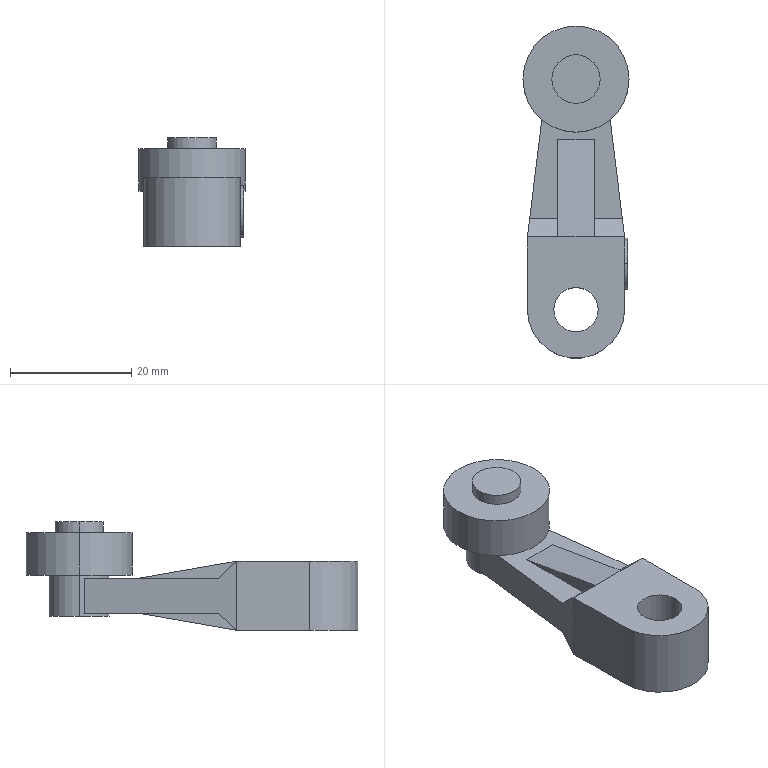Part | SolidWorks | features BaseBody 1 | 1 solid | 34 faces | box 17.5 x 54.75 x 17.9 mm | volume 7250 mm3 | plane 23 | cylinder 11 | commonest cylinder face diameters 7.3 x2 8 x2 8.5 x2 10 x2 17.5 x2 16 x1
STEP:
#1=CARTESIAN_POINT('',(-3.65,0.,0.));
#2=VERTEX_POINT('',#1);
#3=CARTESIAN_POINT('',(3.65,0.,0.));
#4=VERTEX_POINT('',#3);
#5=CARTESIAN_POINT('',(0.,0.,0.));
#6=DIRECTION('',(0.,0.,1.));
#7=DIRECTION('',(1.,0.,0.));
#8=AXIS2_PLACEMENT_3D('',#5,#6,#7);
#9=CIRCLE('',#8,3.65);
#10=EDGE_CURVE('',#2,#4,#9,.T.);
#11=ORIENTED_EDGE('',*,*,#10,.F.);
#12=CARTESIAN_POINT('',(-3.65,0.,11.4));
#13=VERTEX_POINT('',#12);
#14=CARTESIAN_POINT('',(-3.65,0.,0.));
#15=DIRECTION('',(0.,0.,1.));
#16=VECTOR('',#15,1000.);
#17=LINE('',#14,#16);
#18=EDGE_CURVE('',#2,#13,#17,.T.);
#19=ORIENTED_EDGE('',*,*,#18,.T.);
#20=CARTESIAN_POINT('',(3.65,0.,11.4));
#21=VERTEX_POINT('',#20);
#22=CARTESIAN_POINT('',(0.,0.,11.4));
#23=DIRECTION('',(0.,0.,1.));
#24=DIRECTION('',(1.,0.,0.));
#25=AXIS2_PLACEMENT_3D('',#22,#23,#24);
#26=CIRCLE('',#25,3.65);
#27=EDGE_CURVE('',#13,#21,#26,.T.);
#28=ORIENTED_EDGE('',*,*,#27,.T.);
#29=CARTESIAN_POINT('',(3.65,0.,0.));
#30=DIRECTION('',(0.,0.,1.));
#31=VECTOR('',#30,1000.);
#32=LINE('',#29,#31);
#33=EDGE_CURVE('',#4,#21,#32,.T.);
#34=ORIENTED_EDGE('',*,*,#33,.F.);
#35=EDGE_LOOP('',(#11,#19,#28,#34));
#36=FACE_OUTER_BOUND('',#35,.T.);
#37=CARTESIAN_POINT('',(0.,0.,0.));
#38=DIRECTION('',(0.,0.,1.));
#39=DIRECTION('',(1.,0.,0.));
#40=AXIS2_PLACEMENT_3D('',#37,#38,#39);
#41=CYLINDRICAL_SURFACE('',#40,3.65);
#42=ADVANCED_FACE('',(#36),#41,.F.);
#43=CARTESIAN_POINT('',(8.5,7.6,1.45));
#44=VERTEX_POINT('',#43);
#45=CARTESIAN_POINT('',(8.5,7.6,9.95));
#46=VERTEX_POINT('',#45);
#47=CARTESIAN_POINT('',(8.5,7.6,5.7));
#48=DIRECTION('',(1.,0.,0.));
#49=DIRECTION('',(0.,0.,-1.));
#50=AXIS2_PLACEMENT_3D('',#47,#48,#49);
#51=CIRCLE('',#50,4.25);
#52=EDGE_CURVE('',#44,#46,#51,.T.);
#53=ORIENTED_EDGE('',*,*,#52,.F.);
#54=CARTESIAN_POINT('',(8.,7.6,1.45));
#55=VERTEX_POINT('',#54);
#56=CARTESIAN_POINT('',(8.5,7.6,1.45));
#57=DIRECTION('',(-1.,0.,0.));
#58=VECTOR('',#57,1000.);
#59=LINE('',#56,#58);
#60=EDGE_CURVE('',#44,#55,#59,.T.);
#61=ORIENTED_EDGE('',*,*,#60,.T.);
#62=CARTESIAN_POINT('',(8.,7.6,9.95));
#63=VERTEX_POINT('',#62);
#64=CARTESIAN_POINT('',(8.,7.6,5.7));
#65=DIRECTION('',(1.,0.,0.));
#66=DIRECTION('',(0.,0.,-1.));
#67=AXIS2_PLACEMENT_3D('',#64,#65,#66);
#68=CIRCLE('',#67,4.25);
#69=EDGE_CURVE('',#55,#63,#68,.T.);
#70=ORIENTED_EDGE('',*,*,#69,.T.);
#71=CARTESIAN_POINT('',(8.5,7.6,9.95));
#72=DIRECTION('',(-1.,0.,0.));
#73=VECTOR('',#72,1000.);
#74=LINE('',#71,#73);
#75=EDGE_CURVE('',#46,#63,#74,.T.);
#76=ORIENTED_EDGE('',*,*,#75,.F.);
#77=EDGE_LOOP('',(#53,#61,#70,#76));
#78=FACE_OUTER_BOUND('',#77,.T.);
#79=CARTESIAN_POINT('',(8.5,7.6,5.7));
#80=DIRECTION('',(-1.,0.,0.));
#81=DIRECTION('',(0.,0.,1.));
#82=AXIS2_PLACEMENT_3D('',#79,#80,#81);
#83=CYLINDRICAL_SURFACE('',#82,4.25);
#84=ADVANCED_FACE('',(#78),#83,.T.);
#85=CARTESIAN_POINT('',(4.,38.,17.9));
#86=VERTEX_POINT('',#85);
#87=CARTESIAN_POINT('',(-4.,38.,17.9));
#88=VERTEX_POINT('',#87);
#89=CARTESIAN_POINT('',(0.,38.,17.9));
#90=DIRECTION('',(0.,0.,1.));
#91=DIRECTION('',(1.,0.,0.));
#92=AXIS2_PLACEMENT_3D('',#89,#90,#91);
#93=CIRCLE('',#92,4.);
#94=EDGE_CURVE('',#86,#88,#93,.T.);
#95=ORIENTED_EDGE('',*,*,#94,.F.);
#96=CARTESIAN_POINT('',(4.,38.,16.1));
#97=VERTEX_POINT('',#96);
#98=CARTESIAN_POINT('',(4.,38.,17.9));
#99=DIRECTION('',(0.,0.,-1.));
#100=VECTOR('',#99,1000.);
#101=LINE('',#98,#100);
#102=EDGE_CURVE('',#86,#97,#101,.T.);
#103=ORIENTED_EDGE('',*,*,#102,.T.);
#104=CARTESIAN_POINT('',(-4.,38.,16.1));
#105=VERTEX_POINT('',#104);
#106=CARTESIAN_POINT('',(0.,38.,16.1));
#107=DIRECTION('',(0.,0.,1.));
#108=DIRECTION('',(1.,0.,0.));
#109=AXIS2_PLACEMENT_3D('',#106,#107,#108);
#110=CIRCLE('',#109,4.);
#111=EDGE_CURVE('',#97,#105,#110,.T.);
#112=ORIENTED_EDGE('',*,*,#111,.T.);
#113=CARTESIAN_POINT('',(-4.,38.,17.9));
#114=DIRECTION('',(0.,0.,-1.));
#115=VECTOR('',#114,1000.);
#116=LINE('',#113,#115);
#117=EDGE_CURVE('',#88,#105,#116,.T.);
#118=ORIENTED_EDGE('',*,*,#117,.F.);
#119=EDGE_LOOP('',(#95,#103,#112,#118));
#120=FACE_OUTER_BOUND('',#119,.T.);
#121=CARTESIAN_POINT('',(0.,38.,17.9));
#122=DIRECTION('',(0.,0.,-1.));
#123=DIRECTION('',(-1.,0.,0.));
#124=AXIS2_PLACEMENT_3D('',#121,#122,#123);
#125=CYLINDRICAL_SURFACE('',#124,4.);
#126=ADVANCED_FACE('',(#120),#125,.T.);
#127=CARTESIAN_POINT('',(8.75,38.,16.1));
#128=VERTEX_POINT('',#127);
#129=CARTESIAN_POINT('',(-8.75,38.,16.1));
#130=VERTEX_POINT('',#129);
#131=CARTESIAN_POINT('',(0.,38.,16.1));
#132=DIRECTION('',(0.,0.,1.));
#133=DIRECTION('',(1.,0.,0.));
#134=AXIS2_PLACEMENT_3D('',#131,#132,#133);
#135=CIRCLE('',#134,8.75);
#136=EDGE_CURVE('',#128,#130,#135,.T.);
#137=ORIENTED_EDGE('',*,*,#136,.F.);
#138=CARTESIAN_POINT('',(8.75,38.,9.1));
#139=VERTEX_POINT('',#138);
#140=CARTESIAN_POINT('',(8.75,38.,16.1));
#141=DIRECTION('',(0.,0.,-1.));
#142=VECTOR('',#141,1000.);
#143=LINE('',#140,#142);
#144=EDGE_CURVE('',#128,#139,#143,.T.);
#145=ORIENTED_EDGE('',*,*,#144,.T.);
#146=CARTESIAN_POINT('',(-8.75,38.,9.1));
#147=VERTEX_POINT('',#146);
#148=CARTESIAN_POINT('',(0.,38.,9.1));
#149=DIRECTION('',(0.,0.,1.));
#150=DIRECTION('',(1.,0.,0.));
#151=AXIS2_PLACEMENT_3D('',#148,#149,#150);
#152=CIRCLE('',#151,8.75);
#153=EDGE_CURVE('',#139,#147,#152,.T.);
#154=ORIENTED_EDGE('',*,*,#153,.T.);
#155=CARTESIAN_POINT('',(-8.75,38.,16.1));
#156=DIRECTION('',(0.,0.,-1.));
#157=VECTOR('',#156,1000.);
#158=LINE('',#155,#157);
#159=EDGE_CURVE('',#130,#147,#158,.T.);
#160=ORIENTED_EDGE('',*,*,#159,.F.);
#161=EDGE_LOOP('',(#137,#145,#154,#160));
#162=FACE_OUTER_BOUND('',#161,.T.);
#163=CARTESIAN_POINT('',(0.,38.,16.1));
#164=DIRECTION('',(0.,0.,-1.));
#165=DIRECTION('',(-1.,0.,0.));
#166=AXIS2_PLACEMENT_3D('',#163,#164,#165);
#167=CYLINDRICAL_SURFACE('',#166,8.75);
#168=ADVANCED_FACE('',(#162),#167,.T.);
#169=CARTESIAN_POINT('',(-5.,38.,2.3));
#170=VERTEX_POINT('',#169);
#171=CARTESIAN_POINT('',(5.,38.,2.3));
#172=VERTEX_POINT('',#171);
#173=CARTESIAN_POINT('',(0.,38.,2.3));
#174=DIRECTION('',(0.,0.,-1.));
#175=DIRECTION('',(-1.,0.,0.));
#176=AXIS2_PLACEMENT_3D('',#173,#174,#175);
#177=CIRCLE('',#176,5.);
#178=EDGE_CURVE('',#170,#172,#177,.T.);
#179=ORIENTED_EDGE('',*,*,#178,.F.);
#180=CARTESIAN_POINT('',(-5.,38.,9.1));
#181=VERTEX_POINT('',#180);
#182=CARTESIAN_POINT('',(-5.,38.,2.3));
#183=DIRECTION('',(0.,0.,1.));
#184=VECTOR('',#183,1000.);
#185=LINE('',#182,#184);
#186=EDGE_CURVE('',#170,#181,#185,.T.);
#187=ORIENTED_EDGE('',*,*,#186,.T.);
#188=CARTESIAN_POINT('',(5.,38.,9.1));
#189=VERTEX_POINT('',#188);
#190=CARTESIAN_POINT('',(0.,38.,9.1));
#191=DIRECTION('',(0.,0.,1.));
#192=DIRECTION('',(1.,0.,0.));
#193=AXIS2_PLACEMENT_3D('',#190,#191,#192);
#194=CIRCLE('',#193,5.);
#195=EDGE_CURVE('',#189,#181,#194,.T.);
#196=ORIENTED_EDGE('',*,*,#195,.F.);
#197=CARTESIAN_POINT('',(5.,38.,2.3));
#198=DIRECTION('',(0.,0.,1.));
#199=VECTOR('',#198,1000.);
#200=LINE('',#197,#199);
#201=EDGE_CURVE('',#172,#189,#200,.T.);
#202=ORIENTED_EDGE('',*,*,#201,.F.);
#203=EDGE_LOOP('',(#179,#187,#196,#202));
#204=FACE_OUTER_BOUND('',#203,.T.);
#205=CARTESIAN_POINT('',(0.,38.,2.3));
#206=DIRECTION('',(0.,0.,1.));
#207=DIRECTION('',(1.,0.,0.));
#208=AXIS2_PLACEMENT_3D('',#205,#206,#207);
#209=CYLINDRICAL_SURFACE('',#208,5.);
#210=ADVANCED_FACE('',(#204),#209,.T.);
#211=CARTESIAN_POINT('',(8.,0.,0.));
#212=VERTEX_POINT('',#211);
#213=CARTESIAN_POINT('',(8.,12.,0.));
#214=VERTEX_POINT('',#213);
#215=CARTESIAN_POINT('',(8.,0.,0.));
#216=DIRECTION('',(0.,1.,0.));
#217=VECTOR('',#216,1000.);
#218=LINE('',#215,#217);
#219=EDGE_CURVE('',#212,#214,#218,.T.);
#220=ORIENTED_EDGE('',*,*,#219,.T.);
#221=CARTESIAN_POINT('',(8.,12.,11.4));
#222=VERTEX_POINT('',#221);
#223=CARTESIAN_POINT('',(8.,12.,11.4));
#224=DIRECTION('',(0.,0.,1.));
#225=VECTOR('',#224,1000.);
#226=LINE('',#223,#225);
#227=EDGE_CURVE('',#214,#222,#226,.T.);
#228=ORIENTED_EDGE('',*,*,#227,.T.);
#229=CARTESIAN_POINT('',(8.,0.,11.4));
#230=VERTEX_POINT('',#229);
#231=CARTESIAN_POINT('',(8.,0.,11.4));
#232=DIRECTION('',(0.,-1.,0.));
#233=VECTOR('',#232,1000.);
#234=LINE('',#231,#233);
#235=EDGE_CURVE('',#222,#230,#234,.T.);
#236=ORIENTED_EDGE('',*,*,#235,.T.);
#237=CARTESIAN_POINT('',(8.,0.,11.4));
#238=DIRECTION('',(0.,0.,-1.));
#239=VECTOR('',#238,1000.);
#240=LINE('',#237,#239);
#241=EDGE_CURVE('',#230,#212,#240,.T.);
#242=ORIENTED_EDGE('',*,*,#241,.T.);
#243=EDGE_LOOP('',(#220,#228,#236,#242));
#244=FACE_OUTER_BOUND('',#243,.T.);
#245=CARTESIAN_POINT('',(8.,7.6,5.7));
#246=DIRECTION('',(1.,0.,0.));
#247=DIRECTION('',(0.,0.,-1.));
#248=AXIS2_PLACEMENT_3D('',#245,#246,#247);
#249=CIRCLE('',#248,4.25);
#250=EDGE_CURVE('',#63,#55,#249,.T.);
#251=ORIENTED_EDGE('',*,*,#250,.F.);
#252=ORIENTED_EDGE('',*,*,#69,.F.);
#253=EDGE_LOOP('',(#251,#252));
#254=FACE_BOUND('',#253,.T.);
#255=CARTESIAN_POINT('',(8.,38.,11.4));
#256=DIRECTION('',(1.,0.,0.));
#257=DIRECTION('',(0.,0.,-1.));
#258=AXIS2_PLACEMENT_3D('',#255,#256,#257);
#259=PLANE('',#258);
#260=ADVANCED_FACE('',(#244,#254),#259,.T.);
#261=CARTESIAN_POINT('',(0.,38.,16.1));
#262=DIRECTION('',(0.,0.,1.));
#263=DIRECTION('',(1.,0.,0.));
#264=AXIS2_PLACEMENT_3D('',#261,#262,#263);
#265=CIRCLE('',#264,8.75);
#266=EDGE_CURVE('',#130,#128,#265,.T.);
#267=ORIENTED_EDGE('',*,*,#266,.T.);
#268=ORIENTED_EDGE('',*,*,#136,.T.);
#269=EDGE_LOOP('',(#267,#268));
#270=FACE_OUTER_BOUND('',#269,.T.);
#271=CARTESIAN_POINT('',(0.,38.,16.1));
#272=DIRECTION('',(0.,0.,1.));
#273=DIRECTION('',(1.,0.,0.));
#274=AXIS2_PLACEMENT_3D('',#271,#272,#273);
#275=CIRCLE('',#274,4.);
#276=EDGE_CURVE('',#105,#97,#275,.T.);
#277=ORIENTED_EDGE('',*,*,#276,.F.);
#278=ORIENTED_EDGE('',*,*,#111,.F.);
#279=EDGE_LOOP('',(#277,#278));
#280=FACE_BOUND('',#279,.T.);
#281=CARTESIAN_POINT('',(0.,38.,16.1));
#282=DIRECTION('',(0.,0.,1.));
#283=DIRECTION('',(1.,0.,0.));
#284=AXIS2_PLACEMENT_3D('',#281,#282,#283);
#285=PLANE('',#284);
#286=ADVANCED_FACE('',(#270,#280),#285,.T.);
#287=CARTESIAN_POINT('',(-7.632,15.,2.8));
#288=VERTEX_POINT('',#287);
#289=CARTESIAN_POINT('',(-3.,15.,2.8));
#290=VERTEX_POINT('',#289);
#291=CARTESIAN_POINT('',(-8.,15.,2.8));
#292=DIRECTION('',(1.,0.,0.));
#293=VECTOR('',#292,1000.);
#294=LINE('',#291,#293);
#295=EDGE_CURVE('',#288,#290,#294,.T.);
#296=ORIENTED_EDGE('',*,*,#295,.T.);
#297=CARTESIAN_POINT('',(-3.,12.,0.));
#298=VERTEX_POINT('',#297);
#299=CARTESIAN_POINT('',(-3.,15.,2.8));
#300=DIRECTION('',(0.,-0.7311,-0.6823));
#301=VECTOR('',#300,1000.);
#302=LINE('',#299,#301);
#303=EDGE_CURVE('',#290,#298,#302,.T.);
#304=ORIENTED_EDGE('',*,*,#303,.T.);
#305=CARTESIAN_POINT('',(-8.,12.,0.));
#306=VERTEX_POINT('',#305);
#307=CARTESIAN_POINT('',(-8.,12.,0.));
#308=DIRECTION('',(1.,0.,0.));
#309=VECTOR('',#308,1000.);
#310=LINE('',#307,#309);
#311=EDGE_CURVE('',#306,#298,#310,.T.);
#312=ORIENTED_EDGE('',*,*,#311,.F.);
#313=CARTESIAN_POINT('',(-7.635,14.976,2.778));
#314=DIRECTION('',(0.0894,0.7281,0.6796));
#315=VECTOR('',#314,1000.);
#316=LINE('',#313,#315);
#317=EDGE_CURVE('',#306,#288,#316,.T.);
#318=ORIENTED_EDGE('',*,*,#317,.T.);
#319=EDGE_LOOP('',(#296,#304,#312,#318));
#320=FACE_OUTER_BOUND('',#319,.T.);
#321=CARTESIAN_POINT('',(-8.,15.,2.8));
#322=DIRECTION('',(0.,0.6823,-0.7311));
#323=DIRECTION('',(0.,0.7311,0.6823));
#324=AXIS2_PLACEMENT_3D('',#321,#322,#323);
#325=PLANE('',#324);
#326=ADVANCED_FACE('',(#320),#325,.T.);
#327=CARTESIAN_POINT('',(-8.,12.,11.4));
#328=VERTEX_POINT('',#327);
#329=CARTESIAN_POINT('',(-3.,12.,11.4));
#330=VERTEX_POINT('',#329);
#331=CARTESIAN_POINT('',(-8.,12.,11.4));
#332=DIRECTION('',(1.,0.,0.));
#333=VECTOR('',#332,1000.);
#334=LINE('',#331,#333);
#335=EDGE_CURVE('',#328,#330,#334,.T.);
#336=ORIENTED_EDGE('',*,*,#335,.T.);
#337=CARTESIAN_POINT('',(-3.,15.,8.6));
#338=VERTEX_POINT('',#337);
#339=CARTESIAN_POINT('',(-3.,12.,11.4));
#340=DIRECTION('',(0.,0.7311,-0.6823));
#341=VECTOR('',#340,1000.);
#342=LINE('',#339,#341);
#343=EDGE_CURVE('',#330,#338,#342,.T.);
#344=ORIENTED_EDGE('',*,*,#343,.T.);
#345=CARTESIAN_POINT('',(-7.632,15.,8.6));
#346=VERTEX_POINT('',#345);
#347=CARTESIAN_POINT('',(-8.,15.,8.6));
#348=DIRECTION('',(1.,0.,0.));
#349=VECTOR('',#348,1000.);
#350=LINE('',#347,#349);
#351=EDGE_CURVE('',#346,#338,#350,.T.);
#352=ORIENTED_EDGE('',*,*,#351,.F.);
#353=CARTESIAN_POINT('',(-8.,12.,11.4));
#354=DIRECTION('',(-0.0894,-0.7281,0.6796));
#355=VECTOR('',#354,1000.);
#356=LINE('',#353,#355);
#357=EDGE_CURVE('',#346,#328,#356,.T.);
#358=ORIENTED_EDGE('',*,*,#357,.T.);
#359=EDGE_LOOP('',(#336,#344,#352,#358));
#360=FACE_OUTER_BOUND('',#359,.T.);
#361=CARTESIAN_POINT('',(-8.,12.,11.4));
#362=DIRECTION('',(0.,0.6823,0.7311));
#363=DIRECTION('',(0.,-0.7311,0.6823));
#364=AXIS2_PLACEMENT_3D('',#361,#362,#363);
#365=PLANE('',#364);
#366=ADVANCED_FACE('',(#360),#365,.T.);
#367=CARTESIAN_POINT('',(3.,15.,2.8));
#368=VERTEX_POINT('',#367);
#369=CARTESIAN_POINT('',(7.632,15.,2.8));
#370=VERTEX_POINT('',#369);
#371=CARTESIAN_POINT('',(-8.,15.,2.8));
#372=DIRECTION('',(1.,0.,0.));
#373=VECTOR('',#372,1000.);
#374=LINE('',#371,#373);
#375=EDGE_CURVE('',#368,#370,#374,.T.);
#376=ORIENTED_EDGE('',*,*,#375,.F.);
#377=CARTESIAN_POINT('',(3.,28.,2.8));
#378=VERTEX_POINT('',#377);
#379=CARTESIAN_POINT('',(3.,38.,2.8));
#380=DIRECTION('',(0.,-1.,0.));
#381=VECTOR('',#380,1000.);
#382=LINE('',#379,#381);
#383=EDGE_CURVE('',#378,#368,#382,.T.);
#384=ORIENTED_EDGE('',*,*,#383,.F.);
#385=CARTESIAN_POINT('',(-3.,28.,2.8));
#386=VERTEX_POINT('',#385);
#387=CARTESIAN_POINT('',(-8.,28.,2.8));
#388=DIRECTION('',(1.,0.,0.));
#389=VECTOR('',#388,1000.);
#390=LINE('',#387,#389);
#391=EDGE_CURVE('',#386,#378,#390,.T.);
#392=ORIENTED_EDGE('',*,*,#391,.F.);
#393=CARTESIAN_POINT('',(-3.,38.,2.8));
#394=DIRECTION('',(0.,-1.,0.));
#395=VECTOR('',#394,1000.);
#396=LINE('',#393,#395);
#397=EDGE_CURVE('',#386,#290,#396,.T.);
#398=ORIENTED_EDGE('',*,*,#397,.T.);
#399=ORIENTED_EDGE('',*,*,#295,.F.);
#400=CARTESIAN_POINT('',(-4.918,37.099,2.8));
#401=VERTEX_POINT('',#400);
#402=CARTESIAN_POINT('',(-4.855,37.614,2.8));
#403=DIRECTION('',(0.1219,0.9925,0.));
#404=VECTOR('',#403,1000.);
#405=LINE('',#402,#404);
#406=EDGE_CURVE('',#288,#401,#405,.T.);
#407=ORIENTED_EDGE('',*,*,#406,.T.);
#408=CARTESIAN_POINT('',(4.918,37.099,2.8));
#409=VERTEX_POINT('',#408);
#410=CARTESIAN_POINT('',(0.,38.,2.8));
#411=DIRECTION('',(0.,0.,1.));
#412=DIRECTION('',(0.,1.,0.));
#413=AXIS2_PLACEMENT_3D('',#410,#411,#412);
#414=CIRCLE('',#413,5.);
#415=EDGE_CURVE('',#401,#409,#414,.T.);
#416=ORIENTED_EDGE('',*,*,#415,.T.);
#417=CARTESIAN_POINT('',(4.617,39.549,2.8));
#418=DIRECTION('',(0.1219,-0.9925,0.));
#419=VECTOR('',#418,1000.);
#420=LINE('',#417,#419);
#421=EDGE_CURVE('',#409,#370,#420,.T.);
#422=ORIENTED_EDGE('',*,*,#421,.T.);
#423=EDGE_LOOP('',(#376,#384,#392,#398,#399,#407,#416,#422));
#424=FACE_OUTER_BOUND('',#423,.T.);
#425=CARTESIAN_POINT('',(-8.,38.,2.8));
#426=DIRECTION('',(0.,0.,-1.));
#427=DIRECTION('',(0.,1.,0.));
#428=AXIS2_PLACEMENT_3D('',#425,#426,#427);
#429=PLANE('',#428);
#430=ADVANCED_FACE('',(#424),#429,.T.);
#431=CARTESIAN_POINT('',(4.918,37.099,8.6));
#432=VERTEX_POINT('',#431);
#433=CARTESIAN_POINT('',(-4.918,37.099,8.6));
#434=VERTEX_POINT('',#433);
#435=CARTESIAN_POINT('',(0.,38.,8.6));
#436=DIRECTION('',(0.,0.,-1.));
#437=DIRECTION('',(0.,-1.,0.));
#438=AXIS2_PLACEMENT_3D('',#435,#436,#437);
#439=CIRCLE('',#438,5.);
#440=EDGE_CURVE('',#432,#434,#439,.T.);
#441=ORIENTED_EDGE('',*,*,#440,.T.);
#442=CARTESIAN_POINT('',(-7.637,14.955,8.6));
#443=DIRECTION('',(-0.1219,-0.9925,0.));
#444=VECTOR('',#443,1000.);
#445=LINE('',#442,#444);
#446=EDGE_CURVE('',#434,#346,#445,.T.);
#447=ORIENTED_EDGE('',*,*,#446,.T.);
#448=ORIENTED_EDGE('',*,*,#351,.T.);
#449=CARTESIAN_POINT('',(-3.,28.,8.6));
#450=VERTEX_POINT('',#449);
#451=CARTESIAN_POINT('',(-3.,15.,8.6));
#452=DIRECTION('',(0.,1.,0.));
#453=VECTOR('',#452,1000.);
#454=LINE('',#451,#453);
#455=EDGE_CURVE('',#338,#450,#454,.T.);
#456=ORIENTED_EDGE('',*,*,#455,.T.);
#457=CARTESIAN_POINT('',(3.,28.,8.6));
#458=VERTEX_POINT('',#457);
#459=CARTESIAN_POINT('',(-8.,28.,8.6));
#460=DIRECTION('',(-1.,0.,0.));
#461=VECTOR('',#460,1000.);
#462=LINE('',#459,#461);
#463=EDGE_CURVE('',#458,#450,#462,.T.);
#464=ORIENTED_EDGE('',*,*,#463,.F.);
#465=CARTESIAN_POINT('',(3.,15.,8.6));
#466=VERTEX_POINT('',#465);
#467=CARTESIAN_POINT('',(3.,15.,8.6));
#468=DIRECTION('',(0.,1.,0.));
#469=VECTOR('',#468,1000.);
#470=LINE('',#467,#469);
#471=EDGE_CURVE('',#466,#458,#470,.T.);
#472=ORIENTED_EDGE('',*,*,#471,.F.);
#473=CARTESIAN_POINT('',(7.632,15.,8.6));
#474=VERTEX_POINT('',#473);
#475=CARTESIAN_POINT('',(-8.,15.,8.6));
#476=DIRECTION('',(1.,0.,0.));
#477=VECTOR('',#476,1000.);
#478=LINE('',#475,#477);
#479=EDGE_CURVE('',#466,#474,#478,.T.);
#480=ORIENTED_EDGE('',*,*,#479,.T.);
#481=CARTESIAN_POINT('',(7.399,16.891,8.6));
#482=DIRECTION('',(-0.1219,0.9925,0.));
#483=VECTOR('',#482,1000.);
#484=LINE('',#481,#483);
#485=EDGE_CURVE('',#474,#432,#484,.T.);
#486=ORIENTED_EDGE('',*,*,#485,.T.);
#487=EDGE_LOOP('',(#441,#447,#448,#456,#464,#472,#480,#486));
#488=FACE_OUTER_BOUND('',#487,.T.);
#489=CARTESIAN_POINT('',(-8.,15.,8.6));
#490=DIRECTION('',(0.,0.,1.));
#491=DIRECTION('',(0.,-1.,0.));
#492=AXIS2_PLACEMENT_3D('',#489,#490,#491);
#493=PLANE('',#492);
#494=ADVANCED_FACE('',(#488),#493,.T.);
#495=ORIENTED_EDGE('',*,*,#446,.F.);
#496=CARTESIAN_POINT('',(-4.918,37.099,2.3));
#497=DIRECTION('',(0.,0.,-1.));
#498=VECTOR('',#497,1000.);
#499=LINE('',#496,#498);
#500=EDGE_CURVE('',#434,#401,#499,.T.);
#501=ORIENTED_EDGE('',*,*,#500,.T.);
#502=ORIENTED_EDGE('',*,*,#406,.F.);
#503=ORIENTED_EDGE('',*,*,#317,.F.);
#504=CARTESIAN_POINT('',(-8.,12.,11.4));
#505=DIRECTION('',(0.,0.,1.));
#506=VECTOR('',#505,1000.);
#507=LINE('',#504,#506);
#508=EDGE_CURVE('',#306,#328,#507,.T.);
#509=ORIENTED_EDGE('',*,*,#508,.T.);
#510=ORIENTED_EDGE('',*,*,#357,.F.);
#511=EDGE_LOOP('',(#495,#501,#502,#503,#509,#510));
#512=FACE_OUTER_BOUND('',#511,.T.);
#513=CARTESIAN_POINT('',(-4.808,38.,24.3));
#514=DIRECTION('',(-0.9925,0.1219,0.));
#515=DIRECTION('',(-0.1219,-0.9925,0.));
#516=AXIS2_PLACEMENT_3D('',#513,#514,#515);
#517=PLANE('',#516);
#518=ADVANCED_FACE('',(#512),#517,.T.);
#519=ORIENTED_EDGE('',*,*,#421,.F.);
#520=CARTESIAN_POINT('',(4.918,37.099,2.3));
#521=DIRECTION('',(0.,0.,1.));
#522=VECTOR('',#521,1000.);
#523=LINE('',#520,#522);
#524=EDGE_CURVE('',#409,#432,#523,.T.);
#525=ORIENTED_EDGE('',*,*,#524,.T.);
#526=ORIENTED_EDGE('',*,*,#485,.F.);
#527=CARTESIAN_POINT('',(7.872,13.042,10.428));
#528=DIRECTION('',(-0.0894,0.7281,-0.6796));
#529=VECTOR('',#528,1000.);
#530=LINE('',#527,#529);
#531=EDGE_CURVE('',#222,#474,#530,.T.);
#532=ORIENTED_EDGE('',*,*,#531,.F.);
#533=ORIENTED_EDGE('',*,*,#227,.F.);
#534=CARTESIAN_POINT('',(7.507,16.018,3.75));
#535=DIRECTION('',(0.0894,-0.7281,-0.6796));
#536=VECTOR('',#535,1000.);
#537=LINE('',#534,#536);
#538=EDGE_CURVE('',#370,#214,#537,.T.);
#539=ORIENTED_EDGE('',*,*,#538,.F.);
#540=EDGE_LOOP('',(#519,#525,#526,#532,#533,#539));
#541=FACE_OUTER_BOUND('',#540,.T.);
#542=CARTESIAN_POINT('',(4.808,38.,24.3));
#543=DIRECTION('',(0.9925,0.1219,0.));
#544=DIRECTION('',(-0.1219,0.9925,0.));
#545=AXIS2_PLACEMENT_3D('',#542,#543,#544);
#546=PLANE('',#545);
#547=ADVANCED_FACE('',(#541),#546,.T.);
#548=CARTESIAN_POINT('',(3.,12.,0.));
#549=VERTEX_POINT('',#548);
#550=CARTESIAN_POINT('',(3.,15.,2.8));
#551=DIRECTION('',(0.,-0.7311,-0.6823));
#552=VECTOR('',#551,1000.);
#553=LINE('',#550,#552);
#554=EDGE_CURVE('',#368,#549,#553,.T.);
#555=ORIENTED_EDGE('',*,*,#554,.F.);
#556=ORIENTED_EDGE('',*,*,#375,.T.);
#557=ORIENTED_EDGE('',*,*,#538,.T.);
#558=CARTESIAN_POINT('',(-8.,12.,0.));
#559=DIRECTION('',(1.,0.,0.));
#560=VECTOR('',#559,1000.);
#561=LINE('',#558,#560);
#562=EDGE_CURVE('',#549,#214,#561,.T.);
#563=ORIENTED_EDGE('',*,*,#562,.F.);
#564=EDGE_LOOP('',(#555,#556,#557,#563));
#565=FACE_OUTER_BOUND('',#564,.T.);
#566=CARTESIAN_POINT('',(-8.,15.,2.8));
#567=DIRECTION('',(0.,0.6823,-0.7311));
#568=DIRECTION('',(0.,0.7311,0.6823));
#569=AXIS2_PLACEMENT_3D('',#566,#567,#568);
#570=PLANE('',#569);
#571=ADVANCED_FACE('',(#565),#570,.T.);
#572=CARTESIAN_POINT('',(3.,12.,11.4));
#573=VERTEX_POINT('',#572);
#574=CARTESIAN_POINT('',(3.,12.,11.4));
#575=DIRECTION('',(0.,0.7311,-0.6823));
#576=VECTOR('',#575,1000.);
#577=LINE('',#574,#576);
#578=EDGE_CURVE('',#573,#466,#577,.T.);
#579=ORIENTED_EDGE('',*,*,#578,.F.);
#580=CARTESIAN_POINT('',(-8.,12.,11.4));
#581=DIRECTION('',(1.,0.,0.));
#582=VECTOR('',#581,1000.);
#583=LINE('',#580,#582);
#584=EDGE_CURVE('',#573,#222,#583,.T.);
#585=ORIENTED_EDGE('',*,*,#584,.T.);
#586=ORIENTED_EDGE('',*,*,#531,.T.);
#587=ORIENTED_EDGE('',*,*,#479,.F.);
#588=EDGE_LOOP('',(#579,#585,#586,#587));
#589=FACE_OUTER_BOUND('',#588,.T.);
#590=CARTESIAN_POINT('',(-8.,12.,11.4));
#591=DIRECTION('',(0.,0.6823,0.7311));
#592=DIRECTION('',(0.,-0.7311,0.6823));
#593=AXIS2_PLACEMENT_3D('',#590,#591,#592);
#594=PLANE('',#593);
#595=ADVANCED_FACE('',(#589),#594,.T.);
#596=ORIENTED_EDGE('',*,*,#508,.F.);
#597=CARTESIAN_POINT('',(-8.,0.,0.));
#598=VERTEX_POINT('',#597);
#599=CARTESIAN_POINT('',(-8.,0.,0.));
#600=DIRECTION('',(0.,1.,0.));
#601=VECTOR('',#600,1000.);
#602=LINE('',#599,#601);
#603=EDGE_CURVE('',#598,#306,#602,.T.);
#604=ORIENTED_EDGE('',*,*,#603,.F.);
#605=CARTESIAN_POINT('',(-8.,0.,11.4));
#606=VERTEX_POINT('',#605);
#607=CARTESIAN_POINT('',(-8.,0.,11.4));
#608=DIRECTION('',(0.,0.,-1.));
#609=VECTOR('',#608,1000.);
#610=LINE('',#607,#609);
#611=EDGE_CURVE('',#606,#598,#610,.T.);
#612=ORIENTED_EDGE('',*,*,#611,.F.);
#613=CARTESIAN_POINT('',(-8.,0.,11.4));
#614=DIRECTION('',(0.,-1.,0.));
#615=VECTOR('',#614,1000.);
#616=LINE('',#613,#615);
#617=EDGE_CURVE('',#328,#606,#616,.T.);
#618=ORIENTED_EDGE('',*,*,#617,.F.);
#619=EDGE_LOOP('',(#596,#604,#612,#618));
#620=FACE_OUTER_BOUND('',#619,.T.);
#621=CARTESIAN_POINT('',(-8.,38.,11.4));
#622=DIRECTION('',(1.,0.,0.));
#623=DIRECTION('',(0.,0.,-1.));
#624=AXIS2_PLACEMENT_3D('',#621,#622,#623);
#625=PLANE('',#624);
#626=ADVANCED_FACE('',(#620),#625,.F.);
#627=ORIENTED_EDGE('',*,*,#241,.F.);
#628=CARTESIAN_POINT('',(0.,0.,11.4));
#629=DIRECTION('',(0.,0.,1.));
#630=DIRECTION('',(1.,0.,0.));
#631=AXIS2_PLACEMENT_3D('',#628,#629,#630);
#632=CIRCLE('',#631,8.);
#633=EDGE_CURVE('',#606,#230,#632,.T.);
#634=ORIENTED_EDGE('',*,*,#633,.F.);
#635=ORIENTED_EDGE('',*,*,#611,.T.);
#636=CARTESIAN_POINT('',(0.,0.,0.));
#637=DIRECTION('',(0.,0.,1.));
#638=DIRECTION('',(1.,0.,0.));
#639=AXIS2_PLACEMENT_3D('',#636,#637,#638);
#640=CIRCLE('',#639,8.);
#641=EDGE_CURVE('',#598,#212,#640,.T.);
#642=ORIENTED_EDGE('',*,*,#641,.T.);
#643=EDGE_LOOP('',(#627,#634,#635,#642));
#644=FACE_OUTER_BOUND('',#643,.T.);
#645=CARTESIAN_POINT('',(0.,0.,11.4));
#646=DIRECTION('',(0.,0.,-1.));
#647=DIRECTION('',(-1.,0.,0.));
#648=AXIS2_PLACEMENT_3D('',#645,#646,#647);
#649=CYLINDRICAL_SURFACE('',#648,8.);
#650=ADVANCED_FACE('',(#644),#649,.T.);
#651=CARTESIAN_POINT('',(0.,0.,11.4));
#652=DIRECTION('',(0.,0.,1.));
#653=DIRECTION('',(1.,0.,0.));
#654=AXIS2_PLACEMENT_3D('',#651,#652,#653);
#655=CIRCLE('',#654,3.65);
#656=EDGE_CURVE('',#21,#13,#655,.T.);
#657=ORIENTED_EDGE('',*,*,#656,.F.);
#658=ORIENTED_EDGE('',*,*,#27,.F.);
#659=EDGE_LOOP('',(#657,#658));
#660=FACE_BOUND('',#659,.T.);
#661=ORIENTED_EDGE('',*,*,#584,.F.);
#662=CARTESIAN_POINT('',(0.,12.,11.4));
#663=DIRECTION('',(-1.,0.,0.));
#664=VECTOR('',#663,1000.);
#665=LINE('',#662,#664);
#666=EDGE_CURVE('',#573,#330,#665,.T.);
#667=ORIENTED_EDGE('',*,*,#666,.T.);
#668=ORIENTED_EDGE('',*,*,#335,.F.);
#669=ORIENTED_EDGE('',*,*,#617,.T.);
#670=ORIENTED_EDGE('',*,*,#633,.T.);
#671=ORIENTED_EDGE('',*,*,#235,.F.);
#672=EDGE_LOOP('',(#661,#667,#668,#669,#670,#671));
#673=FACE_OUTER_BOUND('',#672,.T.);
#674=CARTESIAN_POINT('',(0.,0.,11.4));
#675=DIRECTION('',(0.,0.,1.));
#676=DIRECTION('',(1.,0.,0.));
#677=AXIS2_PLACEMENT_3D('',#674,#675,#676);
#678=PLANE('',#677);
#679=ADVANCED_FACE('',(#660,#673),#678,.T.);
#680=CARTESIAN_POINT('',(0.,0.,0.));
#681=DIRECTION('',(0.,0.,1.));
#682=DIRECTION('',(1.,0.,0.));
#683=AXIS2_PLACEMENT_3D('',#680,#681,#682);
#684=CIRCLE('',#683,3.65);
#685=EDGE_CURVE('',#4,#2,#684,.T.);
#686=ORIENTED_EDGE('',*,*,#685,.T.);
#687=ORIENTED_EDGE('',*,*,#10,.T.);
#688=EDGE_LOOP('',(#686,#687));
#689=FACE_BOUND('',#688,.T.);
#690=ORIENTED_EDGE('',*,*,#219,.F.);
#691=ORIENTED_EDGE('',*,*,#641,.F.);
#692=ORIENTED_EDGE('',*,*,#603,.T.);
#693=ORIENTED_EDGE('',*,*,#311,.T.);
#694=CARTESIAN_POINT('',(0.,12.,0.));
#695=DIRECTION('',(-1.,0.,0.));
#696=VECTOR('',#695,1000.);
#697=LINE('',#694,#696);
#698=EDGE_CURVE('',#549,#298,#697,.T.);
#699=ORIENTED_EDGE('',*,*,#698,.F.);
#700=ORIENTED_EDGE('',*,*,#562,.T.);
#701=EDGE_LOOP('',(#690,#691,#692,#693,#699,#700));
#702=FACE_OUTER_BOUND('',#701,.T.);
#703=CARTESIAN_POINT('',(0.,0.,0.));
#704=DIRECTION('',(0.,0.,1.));
#705=DIRECTION('',(1.,0.,0.));
#706=AXIS2_PLACEMENT_3D('',#703,#704,#705);
#707=PLANE('',#706);
#708=ADVANCED_FACE('',(#689,#702),#707,.F.);
#709=ORIENTED_EDGE('',*,*,#186,.F.);
#710=CARTESIAN_POINT('',(0.,38.,2.3));
#711=DIRECTION('',(0.,0.,-1.));
#712=DIRECTION('',(-1.,0.,0.));
#713=AXIS2_PLACEMENT_3D('',#710,#711,#712);
#714=CIRCLE('',#713,5.);
#715=EDGE_CURVE('',#172,#170,#714,.T.);
#716=ORIENTED_EDGE('',*,*,#715,.F.);
#717=ORIENTED_EDGE('',*,*,#201,.T.);
#718=CARTESIAN_POINT('',(0.,38.,9.1));
#719=DIRECTION('',(0.,0.,1.));
#720=DIRECTION('',(1.,0.,0.));
#721=AXIS2_PLACEMENT_3D('',#718,#719,#720);
#722=CIRCLE('',#721,5.);
#723=EDGE_CURVE('',#181,#189,#722,.T.);
#724=ORIENTED_EDGE('',*,*,#723,.F.);
#725=EDGE_LOOP('',(#709,#716,#717,#724));
#726=FACE_OUTER_BOUND('',#725,.T.);
#727=ORIENTED_EDGE('',*,*,#500,.F.);
#728=ORIENTED_EDGE('',*,*,#440,.F.);
#729=ORIENTED_EDGE('',*,*,#524,.F.);
#730=ORIENTED_EDGE('',*,*,#415,.F.);
#731=EDGE_LOOP('',(#727,#728,#729,#730));
#732=FACE_BOUND('',#731,.T.);
#733=CARTESIAN_POINT('',(0.,38.,2.3));
#734=DIRECTION('',(0.,0.,1.));
#735=DIRECTION('',(1.,0.,0.));
#736=AXIS2_PLACEMENT_3D('',#733,#734,#735);
#737=CYLINDRICAL_SURFACE('',#736,5.);
#738=ADVANCED_FACE('',(#726,#732),#737,.T.);
#739=ORIENTED_EDGE('',*,*,#715,.T.);
#740=ORIENTED_EDGE('',*,*,#178,.T.);
#741=EDGE_LOOP('',(#739,#740));
#742=FACE_OUTER_BOUND('',#741,.T.);
#743=CARTESIAN_POINT('',(0.,38.,2.3));
#744=DIRECTION('',(0.,0.,-1.));
#745=DIRECTION('',(-1.,0.,0.));
#746=AXIS2_PLACEMENT_3D('',#743,#744,#745);
#747=PLANE('',#746);
#748=ADVANCED_FACE('',(#742),#747,.T.);
#749=CARTESIAN_POINT('',(3.,28.,8.6));
#750=DIRECTION('',(0.,-0.985,0.1724));
#751=VECTOR('',#750,1000.);
#752=LINE('',#749,#751);
#753=EDGE_CURVE('',#458,#573,#752,.T.);
#754=ORIENTED_EDGE('',*,*,#753,.F.);
#755=ORIENTED_EDGE('',*,*,#463,.T.);
#756=CARTESIAN_POINT('',(-3.,28.,8.6));
#757=DIRECTION('',(0.,-0.985,0.1724));
#758=VECTOR('',#757,1000.);
#759=LINE('',#756,#758);
#760=EDGE_CURVE('',#450,#330,#759,.T.);
#761=ORIENTED_EDGE('',*,*,#760,.T.);
#762=ORIENTED_EDGE('',*,*,#666,.F.);
#763=EDGE_LOOP('',(#754,#755,#761,#762));
#764=FACE_OUTER_BOUND('',#763,.T.);
#765=CARTESIAN_POINT('',(0.,28.,8.6));
#766=DIRECTION('',(0.,0.1724,0.985));
#767=DIRECTION('',(0.,-0.985,0.1724));
#768=AXIS2_PLACEMENT_3D('',#765,#766,#767);
#769=PLANE('',#768);
#770=ADVANCED_FACE('',(#764),#769,.T.);
#771=ORIENTED_EDGE('',*,*,#578,.T.);
#772=ORIENTED_EDGE('',*,*,#471,.T.);
#773=ORIENTED_EDGE('',*,*,#753,.T.);
#774=EDGE_LOOP('',(#771,#772,#773));
#775=FACE_OUTER_BOUND('',#774,.T.);
#776=CARTESIAN_POINT('',(3.,17.5,5.7));
#777=DIRECTION('',(1.,0.,0.));
#778=DIRECTION('',(0.,0.,-1.));
#779=AXIS2_PLACEMENT_3D('',#776,#777,#778);
#780=PLANE('',#779);
#781=ADVANCED_FACE('',(#775),#780,.T.);
#782=ORIENTED_EDGE('',*,*,#455,.F.);
#783=ORIENTED_EDGE('',*,*,#343,.F.);
#784=ORIENTED_EDGE('',*,*,#760,.F.);
#785=EDGE_LOOP('',(#782,#783,#784));
#786=FACE_OUTER_BOUND('',#785,.T.);
#787=CARTESIAN_POINT('',(-3.,17.5,5.7));
#788=DIRECTION('',(1.,0.,0.));
#789=DIRECTION('',(0.,0.,-1.));
#790=AXIS2_PLACEMENT_3D('',#787,#788,#789);
#791=PLANE('',#790);
#792=ADVANCED_FACE('',(#786),#791,.F.);
#793=ORIENTED_EDGE('',*,*,#383,.T.);
#794=ORIENTED_EDGE('',*,*,#554,.T.);
#795=CARTESIAN_POINT('',(3.,28.,2.8));
#796=DIRECTION('',(0.,-0.985,-0.1724));
#797=VECTOR('',#796,1000.);
#798=LINE('',#795,#797);
#799=EDGE_CURVE('',#378,#549,#798,.T.);
#800=ORIENTED_EDGE('',*,*,#799,.F.);
#801=EDGE_LOOP('',(#793,#794,#800));
#802=FACE_OUTER_BOUND('',#801,.T.);
#803=CARTESIAN_POINT('',(3.,17.5,5.7));
#804=DIRECTION('',(1.,0.,0.));
#805=DIRECTION('',(0.,0.,-1.));
#806=AXIS2_PLACEMENT_3D('',#803,#804,#805);
#807=PLANE('',#806);
#808=ADVANCED_FACE('',(#802),#807,.T.);
#809=ORIENTED_EDGE('',*,*,#397,.F.);
#810=CARTESIAN_POINT('',(-3.,28.,2.8));
#811=DIRECTION('',(0.,-0.985,-0.1724));
#812=VECTOR('',#811,1000.);
#813=LINE('',#810,#812);
#814=EDGE_CURVE('',#386,#298,#813,.T.);
#815=ORIENTED_EDGE('',*,*,#814,.T.);
#816=ORIENTED_EDGE('',*,*,#303,.F.);
#817=EDGE_LOOP('',(#809,#815,#816));
#818=FACE_OUTER_BOUND('',#817,.T.);
#819=CARTESIAN_POINT('',(-3.,17.5,5.7));
#820=DIRECTION('',(1.,0.,0.));
#821=DIRECTION('',(0.,0.,-1.));
#822=AXIS2_PLACEMENT_3D('',#819,#820,#821);
#823=PLANE('',#822);
#824=ADVANCED_FACE('',(#818),#823,.F.);
#825=ORIENTED_EDGE('',*,*,#814,.F.);
#826=ORIENTED_EDGE('',*,*,#391,.T.);
#827=ORIENTED_EDGE('',*,*,#799,.T.);
#828=ORIENTED_EDGE('',*,*,#698,.T.);
#829=EDGE_LOOP('',(#825,#826,#827,#828));
#830=FACE_OUTER_BOUND('',#829,.T.);
#831=CARTESIAN_POINT('',(0.,28.,2.8));
#832=DIRECTION('',(0.,-0.1724,0.985));
#833=DIRECTION('',(0.,-0.985,-0.1724));
#834=AXIS2_PLACEMENT_3D('',#831,#832,#833);
#835=PLANE('',#834);
#836=ADVANCED_FACE('',(#830),#835,.F.);
#837=CARTESIAN_POINT('',(0.,38.,9.1));
#838=DIRECTION('',(0.,0.,1.));
#839=DIRECTION('',(1.,0.,0.));
#840=AXIS2_PLACEMENT_3D('',#837,#838,#839);
#841=CIRCLE('',#840,8.75);
#842=EDGE_CURVE('',#147,#139,#841,.T.);
#843=ORIENTED_EDGE('',*,*,#842,.F.);
#844=ORIENTED_EDGE('',*,*,#153,.F.);
#845=EDGE_LOOP('',(#843,#844));
#846=FACE_OUTER_BOUND('',#845,.T.);
#847=ORIENTED_EDGE('',*,*,#195,.T.);
#848=ORIENTED_EDGE('',*,*,#723,.T.);
#849=EDGE_LOOP('',(#847,#848));
#850=FACE_BOUND('',#849,.T.);
#851=CARTESIAN_POINT('',(0.,38.,9.1));
#852=DIRECTION('',(0.,0.,1.));
#853=DIRECTION('',(1.,0.,0.));
#854=AXIS2_PLACEMENT_3D('',#851,#852,#853);
#855=PLANE('',#854);
#856=ADVANCED_FACE('',(#846,#850),#855,.F.);
#857=ORIENTED_EDGE('',*,*,#144,.F.);
#858=ORIENTED_EDGE('',*,*,#266,.F.);
#859=ORIENTED_EDGE('',*,*,#159,.T.);
#860=ORIENTED_EDGE('',*,*,#842,.T.);
#861=EDGE_LOOP('',(#857,#858,#859,#860));
#862=FACE_OUTER_BOUND('',#861,.T.);
#863=CARTESIAN_POINT('',(0.,38.,16.1));
#864=DIRECTION('',(0.,0.,-1.));
#865=DIRECTION('',(-1.,0.,0.));
#866=AXIS2_PLACEMENT_3D('',#863,#864,#865);
#867=CYLINDRICAL_SURFACE('',#866,8.75);
#868=ADVANCED_FACE('',(#862),#867,.T.);
#869=ORIENTED_EDGE('',*,*,#102,.F.);
#870=CARTESIAN_POINT('',(0.,38.,17.9));
#871=DIRECTION('',(0.,0.,1.));
#872=DIRECTION('',(1.,0.,0.));
#873=AXIS2_PLACEMENT_3D('',#870,#871,#872);
#874=CIRCLE('',#873,4.);
#875=EDGE_CURVE('',#88,#86,#874,.T.);
#876=ORIENTED_EDGE('',*,*,#875,.F.);
#877=ORIENTED_EDGE('',*,*,#117,.T.);
#878=ORIENTED_EDGE('',*,*,#276,.T.);
#879=EDGE_LOOP('',(#869,#876,#877,#878));
#880=FACE_OUTER_BOUND('',#879,.T.);
#881=CARTESIAN_POINT('',(0.,38.,17.9));
#882=DIRECTION('',(0.,0.,-1.));
#883=DIRECTION('',(-1.,0.,0.));
#884=AXIS2_PLACEMENT_3D('',#881,#882,#883);
#885=CYLINDRICAL_SURFACE('',#884,4.);
#886=ADVANCED_FACE('',(#880),#885,.T.);
#887=ORIENTED_EDGE('',*,*,#875,.T.);
#888=ORIENTED_EDGE('',*,*,#94,.T.);
#889=EDGE_LOOP('',(#887,#888));
#890=FACE_OUTER_BOUND('',#889,.T.);
#891=CARTESIAN_POINT('',(0.,38.,17.9));
#892=DIRECTION('',(0.,0.,1.));
#893=DIRECTION('',(1.,0.,0.));
#894=AXIS2_PLACEMENT_3D('',#891,#892,#893);
#895=PLANE('',#894);
#896=ADVANCED_FACE('',(#890),#895,.T.);
#897=ORIENTED_EDGE('',*,*,#60,.F.);
#898=CARTESIAN_POINT('',(8.5,7.6,5.7));
#899=DIRECTION('',(1.,0.,0.));
#900=DIRECTION('',(0.,0.,-1.));
#901=AXIS2_PLACEMENT_3D('',#898,#899,#900);
#902=CIRCLE('',#901,4.25);
#903=EDGE_CURVE('',#46,#44,#902,.T.);
#904=ORIENTED_EDGE('',*,*,#903,.F.);
#905=ORIENTED_EDGE('',*,*,#75,.T.);
#906=ORIENTED_EDGE('',*,*,#250,.T.);
#907=EDGE_LOOP('',(#897,#904,#905,#906));
#908=FACE_OUTER_BOUND('',#907,.T.);
#909=CARTESIAN_POINT('',(8.5,7.6,5.7));
#910=DIRECTION('',(-1.,0.,0.));
#911=DIRECTION('',(0.,0.,1.));
#912=AXIS2_PLACEMENT_3D('',#909,#910,#911);
#913=CYLINDRICAL_SURFACE('',#912,4.25);
#914=ADVANCED_FACE('',(#908),#913,.T.);
#915=ORIENTED_EDGE('',*,*,#903,.T.);
#916=ORIENTED_EDGE('',*,*,#52,.T.);
#917=EDGE_LOOP('',(#915,#916));
#918=FACE_OUTER_BOUND('',#917,.T.);
#919=CARTESIAN_POINT('',(8.5,7.6,5.7));
#920=DIRECTION('',(1.,0.,0.));
#921=DIRECTION('',(0.,0.,-1.));
#922=AXIS2_PLACEMENT_3D('',#919,#920,#921);
#923=PLANE('',#922);
#924=ADVANCED_FACE('',(#918),#923,.T.);
#925=ORIENTED_EDGE('',*,*,#18,.F.);
#926=ORIENTED_EDGE('',*,*,#685,.F.);
#927=ORIENTED_EDGE('',*,*,#33,.T.);
#928=ORIENTED_EDGE('',*,*,#656,.T.);
#929=EDGE_LOOP('',(#925,#926,#927,#928));
#930=FACE_OUTER_BOUND('',#929,.T.);
#931=CARTESIAN_POINT('',(0.,0.,0.));
#932=DIRECTION('',(0.,0.,1.));
#933=DIRECTION('',(1.,0.,0.));
#934=AXIS2_PLACEMENT_3D('',#931,#932,#933);
#935=CYLINDRICAL_SURFACE('',#934,3.65);
#936=ADVANCED_FACE('',(#930),#935,.F.);
#937=CLOSED_SHELL('',(#42,#84,#126,#168,#210,#260,#286,#326,#366,#430,#494,#518,#547,#571,#595,#626,#650,#679,#708,#738,#748,#770,#781,#792,#808,#824,#836,#856,#868,#886,#896,#914,#924,#936));
#938=MANIFOLD_SOLID_BREP('',#937);
#939=CARTESIAN_POINT('',(0.,0.,0.));
#940=DIRECTION('',(0.,0.,1.));
#941=DIRECTION('',(1.,0.,0.));
#942=AXIS2_PLACEMENT_3D('',#939,#940,#941);
#943=(LENGTH_UNIT()NAMED_UNIT(*)SI_UNIT(.MILLI.,.METRE.));
#944=UNCERTAINTY_MEASURE_WITH_UNIT(LENGTH_MEASURE(0.00001),#943,'','');
#945=(NAMED_UNIT(*)PLANE_ANGLE_UNIT()SI_UNIT($,.RADIAN.));
#946=(NAMED_UNIT(*)SI_UNIT($,.STERADIAN.)SOLID_ANGLE_UNIT());
#947=(GEOMETRIC_REPRESENTATION_CONTEXT(3)GLOBAL_UNCERTAINTY_ASSIGNED_CONTEXT((#944))GLOBAL_UNIT_ASSIGNED_CONTEXT((#943,#945,#946))REPRESENTATION_CONTEXT('',''));
#948=ADVANCED_BREP_SHAPE_REPRESENTATION('',(#938,#942),#947);